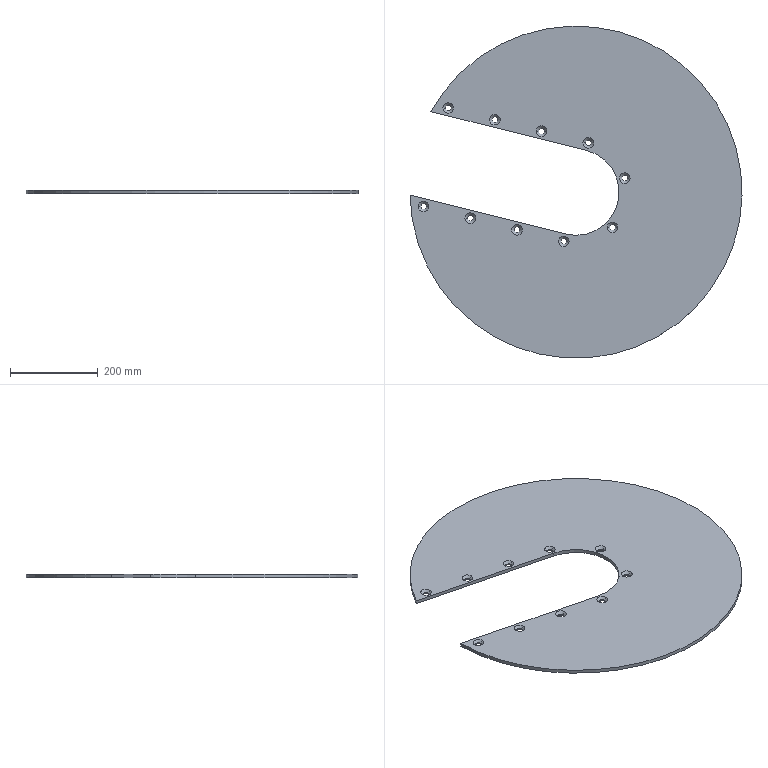Part | SolidWorks | features Extrusion 1, HoleWzd 1 | 1 solid | 46 faces | box 758.937 x 759 x 8 mm | volume 2886950 mm3 | cylinder 22 | cone 20 | plane 4 | commonest cylinder face diameters 13.5 x20 197 x1 759 x1
STEP:
#1=CARTESIAN_POINT('',(-298.885,192.389,2.55));
#2=VERTEX_POINT('',#1);
#3=CARTESIAN_POINT('',(-285.385,192.389,2.55));
#4=VERTEX_POINT('',#3);
#5=CARTESIAN_POINT('',(-292.135,192.389,2.55));
#6=DIRECTION('',(0.,0.,1.));
#7=DIRECTION('',(1.,0.,0.));
#8=AXIS2_PLACEMENT_3D('',#5,#6,#7);
#9=CIRCLE('',#8,6.75);
#10=EDGE_CURVE('',#2,#4,#9,.T.);
#11=ORIENTED_EDGE('',*,*,#10,.F.);
#12=CARTESIAN_POINT('',(-304.335,192.389,8.));
#13=VERTEX_POINT('',#12);
#14=CARTESIAN_POINT('',(-304.335,192.389,8.));
#15=DIRECTION('',(-0.7071,0.,0.7071));
#16=VECTOR('',#15,1000.);
#17=LINE('',#14,#16);
#18=EDGE_CURVE('',#2,#13,#17,.T.);
#19=ORIENTED_EDGE('',*,*,#18,.T.);
#20=CARTESIAN_POINT('',(-279.935,192.389,8.));
#21=VERTEX_POINT('',#20);
#22=CARTESIAN_POINT('',(-292.135,192.389,8.));
#23=DIRECTION('',(0.,0.,1.));
#24=DIRECTION('',(1.,0.,0.));
#25=AXIS2_PLACEMENT_3D('',#22,#23,#24);
#26=CIRCLE('',#25,12.2);
#27=EDGE_CURVE('',#13,#21,#26,.T.);
#28=ORIENTED_EDGE('',*,*,#27,.T.);
#29=CARTESIAN_POINT('',(-279.935,192.389,8.));
#30=DIRECTION('',(0.7071,0.,0.7071));
#31=VECTOR('',#30,1000.);
#32=LINE('',#29,#31);
#33=EDGE_CURVE('',#4,#21,#32,.T.);
#34=ORIENTED_EDGE('',*,*,#33,.F.);
#35=EDGE_LOOP('',(#11,#19,#28,#34));
#36=FACE_OUTER_BOUND('',#35,.T.);
#37=CARTESIAN_POINT('',(-292.135,192.389,8.));
#38=DIRECTION('',(0.,0.,1.));
#39=DIRECTION('',(1.,0.,0.));
#40=AXIS2_PLACEMENT_3D('',#37,#38,#39);
#41=CONICAL_SURFACE('',#40,12.2,0.7854);
#42=ADVANCED_FACE('',(#36),#41,.F.);
#43=CARTESIAN_POINT('',(-298.885,192.389,0.));
#44=VERTEX_POINT('',#43);
#45=CARTESIAN_POINT('',(-285.385,192.389,0.));
#46=VERTEX_POINT('',#45);
#47=CARTESIAN_POINT('',(-292.135,192.389,0.));
#48=DIRECTION('',(0.,0.,1.));
#49=DIRECTION('',(1.,0.,0.));
#50=AXIS2_PLACEMENT_3D('',#47,#48,#49);
#51=CIRCLE('',#50,6.75);
#52=EDGE_CURVE('',#44,#46,#51,.T.);
#53=ORIENTED_EDGE('',*,*,#52,.F.);
#54=CARTESIAN_POINT('',(-298.885,192.389,8.));
#55=DIRECTION('',(0.,0.,1.));
#56=VECTOR('',#55,1000.);
#57=LINE('',#54,#56);
#58=EDGE_CURVE('',#44,#2,#57,.T.);
#59=ORIENTED_EDGE('',*,*,#58,.T.);
#60=ORIENTED_EDGE('',*,*,#10,.T.);
#61=CARTESIAN_POINT('',(-285.385,192.389,8.));
#62=DIRECTION('',(0.,0.,1.));
#63=VECTOR('',#62,1000.);
#64=LINE('',#61,#63);
#65=EDGE_CURVE('',#46,#4,#64,.T.);
#66=ORIENTED_EDGE('',*,*,#65,.F.);
#67=EDGE_LOOP('',(#53,#59,#60,#66));
#68=FACE_OUTER_BOUND('',#67,.T.);
#69=CARTESIAN_POINT('',(-292.135,192.389,8.));
#70=DIRECTION('',(0.,0.,1.));
#71=DIRECTION('',(1.,0.,0.));
#72=AXIS2_PLACEMENT_3D('',#69,#70,#71);
#73=CYLINDRICAL_SURFACE('',#72,6.75);
#74=ADVANCED_FACE('',(#68),#73,.F.);
#75=CARTESIAN_POINT('',(-192.152,165.777,2.55));
#76=VERTEX_POINT('',#75);
#77=CARTESIAN_POINT('',(-178.652,165.777,2.55));
#78=VERTEX_POINT('',#77);
#79=CARTESIAN_POINT('',(-185.402,165.777,2.55));
#80=DIRECTION('',(0.,0.,1.));
#81=DIRECTION('',(1.,0.,0.));
#82=AXIS2_PLACEMENT_3D('',#79,#80,#81);
#83=CIRCLE('',#82,6.75);
#84=EDGE_CURVE('',#76,#78,#83,.T.);
#85=ORIENTED_EDGE('',*,*,#84,.F.);
#86=CARTESIAN_POINT('',(-197.602,165.777,8.));
#87=VERTEX_POINT('',#86);
#88=CARTESIAN_POINT('',(-197.602,165.777,8.));
#89=DIRECTION('',(-0.7071,0.,0.7071));
#90=VECTOR('',#89,1000.);
#91=LINE('',#88,#90);
#92=EDGE_CURVE('',#76,#87,#91,.T.);
#93=ORIENTED_EDGE('',*,*,#92,.T.);
#94=CARTESIAN_POINT('',(-173.202,165.777,8.));
#95=VERTEX_POINT('',#94);
#96=CARTESIAN_POINT('',(-185.402,165.777,8.));
#97=DIRECTION('',(0.,0.,1.));
#98=DIRECTION('',(1.,0.,0.));
#99=AXIS2_PLACEMENT_3D('',#96,#97,#98);
#100=CIRCLE('',#99,12.2);
#101=EDGE_CURVE('',#87,#95,#100,.T.);
#102=ORIENTED_EDGE('',*,*,#101,.T.);
#103=CARTESIAN_POINT('',(-173.202,165.777,8.));
#104=DIRECTION('',(0.7071,0.,0.7071));
#105=VECTOR('',#104,1000.);
#106=LINE('',#103,#105);
#107=EDGE_CURVE('',#78,#95,#106,.T.);
#108=ORIENTED_EDGE('',*,*,#107,.F.);
#109=EDGE_LOOP('',(#85,#93,#102,#108));
#110=FACE_OUTER_BOUND('',#109,.T.);
#111=CARTESIAN_POINT('',(-185.402,165.777,8.));
#112=DIRECTION('',(0.,0.,1.));
#113=DIRECTION('',(1.,0.,0.));
#114=AXIS2_PLACEMENT_3D('',#111,#112,#113);
#115=CONICAL_SURFACE('',#114,12.2,0.7854);
#116=ADVANCED_FACE('',(#110),#115,.F.);
#117=CARTESIAN_POINT('',(-192.152,165.777,0.));
#118=VERTEX_POINT('',#117);
#119=CARTESIAN_POINT('',(-178.652,165.777,0.));
#120=VERTEX_POINT('',#119);
#121=CARTESIAN_POINT('',(-185.402,165.777,0.));
#122=DIRECTION('',(0.,0.,1.));
#123=DIRECTION('',(1.,0.,0.));
#124=AXIS2_PLACEMENT_3D('',#121,#122,#123);
#125=CIRCLE('',#124,6.75);
#126=EDGE_CURVE('',#118,#120,#125,.T.);
#127=ORIENTED_EDGE('',*,*,#126,.F.);
#128=CARTESIAN_POINT('',(-192.152,165.777,8.));
#129=DIRECTION('',(0.,0.,1.));
#130=VECTOR('',#129,1000.);
#131=LINE('',#128,#130);
#132=EDGE_CURVE('',#118,#76,#131,.T.);
#133=ORIENTED_EDGE('',*,*,#132,.T.);
#134=ORIENTED_EDGE('',*,*,#84,.T.);
#135=CARTESIAN_POINT('',(-178.652,165.777,8.));
#136=DIRECTION('',(0.,0.,1.));
#137=VECTOR('',#136,1000.);
#138=LINE('',#135,#137);
#139=EDGE_CURVE('',#120,#78,#138,.T.);
#140=ORIENTED_EDGE('',*,*,#139,.F.);
#141=EDGE_LOOP('',(#127,#133,#134,#140));
#142=FACE_OUTER_BOUND('',#141,.T.);
#143=CARTESIAN_POINT('',(-185.402,165.777,8.));
#144=DIRECTION('',(0.,0.,1.));
#145=DIRECTION('',(1.,0.,0.));
#146=AXIS2_PLACEMENT_3D('',#143,#144,#145);
#147=CYLINDRICAL_SURFACE('',#146,6.75);
#148=ADVANCED_FACE('',(#142),#147,.F.);
#149=CARTESIAN_POINT('',(-85.42,139.166,2.55));
#150=VERTEX_POINT('',#149);
#151=CARTESIAN_POINT('',(-71.92,139.166,2.55));
#152=VERTEX_POINT('',#151);
#153=CARTESIAN_POINT('',(-78.67,139.166,2.55));
#154=DIRECTION('',(0.,0.,1.));
#155=DIRECTION('',(1.,0.,0.));
#156=AXIS2_PLACEMENT_3D('',#153,#154,#155);
#157=CIRCLE('',#156,6.75);
#158=EDGE_CURVE('',#150,#152,#157,.T.);
#159=ORIENTED_EDGE('',*,*,#158,.F.);
#160=CARTESIAN_POINT('',(-90.87,139.166,8.));
#161=VERTEX_POINT('',#160);
#162=CARTESIAN_POINT('',(-90.87,139.166,8.));
#163=DIRECTION('',(-0.7071,0.,0.7071));
#164=VECTOR('',#163,1000.);
#165=LINE('',#162,#164);
#166=EDGE_CURVE('',#150,#161,#165,.T.);
#167=ORIENTED_EDGE('',*,*,#166,.T.);
#168=CARTESIAN_POINT('',(-66.47,139.166,8.));
#169=VERTEX_POINT('',#168);
#170=CARTESIAN_POINT('',(-78.67,139.166,8.));
#171=DIRECTION('',(0.,0.,1.));
#172=DIRECTION('',(1.,0.,0.));
#173=AXIS2_PLACEMENT_3D('',#170,#171,#172);
#174=CIRCLE('',#173,12.2);
#175=EDGE_CURVE('',#161,#169,#174,.T.);
#176=ORIENTED_EDGE('',*,*,#175,.T.);
#177=CARTESIAN_POINT('',(-66.47,139.166,8.));
#178=DIRECTION('',(0.7071,0.,0.7071));
#179=VECTOR('',#178,1000.);
#180=LINE('',#177,#179);
#181=EDGE_CURVE('',#152,#169,#180,.T.);
#182=ORIENTED_EDGE('',*,*,#181,.F.);
#183=EDGE_LOOP('',(#159,#167,#176,#182));
#184=FACE_OUTER_BOUND('',#183,.T.);
#185=CARTESIAN_POINT('',(-78.67,139.166,8.));
#186=DIRECTION('',(0.,0.,1.));
#187=DIRECTION('',(1.,0.,0.));
#188=AXIS2_PLACEMENT_3D('',#185,#186,#187);
#189=CONICAL_SURFACE('',#188,12.2,0.7854);
#190=ADVANCED_FACE('',(#184),#189,.F.);
#191=CARTESIAN_POINT('',(-85.42,139.166,0.));
#192=VERTEX_POINT('',#191);
#193=CARTESIAN_POINT('',(-71.92,139.166,0.));
#194=VERTEX_POINT('',#193);
#195=CARTESIAN_POINT('',(-78.67,139.166,0.));
#196=DIRECTION('',(0.,0.,1.));
#197=DIRECTION('',(1.,0.,0.));
#198=AXIS2_PLACEMENT_3D('',#195,#196,#197);
#199=CIRCLE('',#198,6.75);
#200=EDGE_CURVE('',#192,#194,#199,.T.);
#201=ORIENTED_EDGE('',*,*,#200,.F.);
#202=CARTESIAN_POINT('',(-85.42,139.166,8.));
#203=DIRECTION('',(0.,0.,1.));
#204=VECTOR('',#203,1000.);
#205=LINE('',#202,#204);
#206=EDGE_CURVE('',#192,#150,#205,.T.);
#207=ORIENTED_EDGE('',*,*,#206,.T.);
#208=ORIENTED_EDGE('',*,*,#158,.T.);
#209=CARTESIAN_POINT('',(-71.92,139.166,8.));
#210=DIRECTION('',(0.,0.,1.));
#211=VECTOR('',#210,1000.);
#212=LINE('',#209,#211);
#213=EDGE_CURVE('',#194,#152,#212,.T.);
#214=ORIENTED_EDGE('',*,*,#213,.F.);
#215=EDGE_LOOP('',(#201,#207,#208,#214));
#216=FACE_OUTER_BOUND('',#215,.T.);
#217=CARTESIAN_POINT('',(-78.67,139.166,8.));
#218=DIRECTION('',(0.,0.,1.));
#219=DIRECTION('',(1.,0.,0.));
#220=AXIS2_PLACEMENT_3D('',#217,#218,#219);
#221=CYLINDRICAL_SURFACE('',#220,6.75);
#222=ADVANCED_FACE('',(#216),#221,.F.);
#223=CARTESIAN_POINT('',(21.313,112.554,2.55));
#224=VERTEX_POINT('',#223);
#225=CARTESIAN_POINT('',(34.813,112.554,2.55));
#226=VERTEX_POINT('',#225);
#227=CARTESIAN_POINT('',(28.063,112.554,2.55));
#228=DIRECTION('',(0.,0.,1.));
#229=DIRECTION('',(1.,0.,0.));
#230=AXIS2_PLACEMENT_3D('',#227,#228,#229);
#231=CIRCLE('',#230,6.75);
#232=EDGE_CURVE('',#224,#226,#231,.T.);
#233=ORIENTED_EDGE('',*,*,#232,.F.);
#234=CARTESIAN_POINT('',(15.863,112.554,8.));
#235=VERTEX_POINT('',#234);
#236=CARTESIAN_POINT('',(15.863,112.554,8.));
#237=DIRECTION('',(-0.7071,0.,0.7071));
#238=VECTOR('',#237,1000.);
#239=LINE('',#236,#238);
#240=EDGE_CURVE('',#224,#235,#239,.T.);
#241=ORIENTED_EDGE('',*,*,#240,.T.);
#242=CARTESIAN_POINT('',(40.263,112.554,8.));
#243=VERTEX_POINT('',#242);
#244=CARTESIAN_POINT('',(28.063,112.554,8.));
#245=DIRECTION('',(0.,0.,1.));
#246=DIRECTION('',(1.,0.,0.));
#247=AXIS2_PLACEMENT_3D('',#244,#245,#246);
#248=CIRCLE('',#247,12.2);
#249=EDGE_CURVE('',#235,#243,#248,.T.);
#250=ORIENTED_EDGE('',*,*,#249,.T.);
#251=CARTESIAN_POINT('',(40.263,112.554,8.));
#252=DIRECTION('',(0.7071,0.,0.7071));
#253=VECTOR('',#252,1000.);
#254=LINE('',#251,#253);
#255=EDGE_CURVE('',#226,#243,#254,.T.);
#256=ORIENTED_EDGE('',*,*,#255,.F.);
#257=EDGE_LOOP('',(#233,#241,#250,#256));
#258=FACE_OUTER_BOUND('',#257,.T.);
#259=CARTESIAN_POINT('',(28.063,112.554,8.));
#260=DIRECTION('',(0.,0.,1.));
#261=DIRECTION('',(1.,0.,0.));
#262=AXIS2_PLACEMENT_3D('',#259,#260,#261);
#263=CONICAL_SURFACE('',#262,12.2,0.7854);
#264=ADVANCED_FACE('',(#258),#263,.F.);
#265=CARTESIAN_POINT('',(21.313,112.554,0.));
#266=VERTEX_POINT('',#265);
#267=CARTESIAN_POINT('',(34.813,112.554,0.));
#268=VERTEX_POINT('',#267);
#269=CARTESIAN_POINT('',(28.063,112.554,0.));
#270=DIRECTION('',(0.,0.,1.));
#271=DIRECTION('',(1.,0.,0.));
#272=AXIS2_PLACEMENT_3D('',#269,#270,#271);
#273=CIRCLE('',#272,6.75);
#274=EDGE_CURVE('',#266,#268,#273,.T.);
#275=ORIENTED_EDGE('',*,*,#274,.F.);
#276=CARTESIAN_POINT('',(21.313,112.554,8.));
#277=DIRECTION('',(0.,0.,1.));
#278=VECTOR('',#277,1000.);
#279=LINE('',#276,#278);
#280=EDGE_CURVE('',#266,#224,#279,.T.);
#281=ORIENTED_EDGE('',*,*,#280,.T.);
#282=ORIENTED_EDGE('',*,*,#232,.T.);
#283=CARTESIAN_POINT('',(34.813,112.554,8.));
#284=DIRECTION('',(0.,0.,1.));
#285=VECTOR('',#284,1000.);
#286=LINE('',#283,#285);
#287=EDGE_CURVE('',#268,#226,#286,.T.);
#288=ORIENTED_EDGE('',*,*,#287,.F.);
#289=EDGE_LOOP('',(#275,#281,#282,#288));
#290=FACE_OUTER_BOUND('',#289,.T.);
#291=CARTESIAN_POINT('',(28.063,112.554,8.));
#292=DIRECTION('',(0.,0.,1.));
#293=DIRECTION('',(1.,0.,0.));
#294=AXIS2_PLACEMENT_3D('',#291,#292,#293);
#295=CYLINDRICAL_SURFACE('',#294,6.75);
#296=ADVANCED_FACE('',(#290),#295,.F.);
#297=CARTESIAN_POINT('',(104.756,31.974,2.55));
#298=VERTEX_POINT('',#297);
#299=CARTESIAN_POINT('',(118.256,31.974,2.55));
#300=VERTEX_POINT('',#299);
#301=CARTESIAN_POINT('',(111.506,31.974,2.55));
#302=DIRECTION('',(0.,0.,1.));
#303=DIRECTION('',(1.,0.,0.));
#304=AXIS2_PLACEMENT_3D('',#301,#302,#303);
#305=CIRCLE('',#304,6.75);
#306=EDGE_CURVE('',#298,#300,#305,.T.);
#307=ORIENTED_EDGE('',*,*,#306,.F.);
#308=CARTESIAN_POINT('',(99.306,31.974,8.));
#309=VERTEX_POINT('',#308);
#310=CARTESIAN_POINT('',(99.306,31.974,8.));
#311=DIRECTION('',(-0.7071,0.,0.7071));
#312=VECTOR('',#311,1000.);
#313=LINE('',#310,#312);
#314=EDGE_CURVE('',#298,#309,#313,.T.);
#315=ORIENTED_EDGE('',*,*,#314,.T.);
#316=CARTESIAN_POINT('',(123.706,31.974,8.));
#317=VERTEX_POINT('',#316);
#318=CARTESIAN_POINT('',(111.506,31.974,8.));
#319=DIRECTION('',(0.,0.,1.));
#320=DIRECTION('',(1.,0.,0.));
#321=AXIS2_PLACEMENT_3D('',#318,#319,#320);
#322=CIRCLE('',#321,12.2);
#323=EDGE_CURVE('',#309,#317,#322,.T.);
#324=ORIENTED_EDGE('',*,*,#323,.T.);
#325=CARTESIAN_POINT('',(123.706,31.974,8.));
#326=DIRECTION('',(0.7071,0.,0.7071));
#327=VECTOR('',#326,1000.);
#328=LINE('',#325,#327);
#329=EDGE_CURVE('',#300,#317,#328,.T.);
#330=ORIENTED_EDGE('',*,*,#329,.F.);
#331=EDGE_LOOP('',(#307,#315,#324,#330));
#332=FACE_OUTER_BOUND('',#331,.T.);
#333=CARTESIAN_POINT('',(111.506,31.974,8.));
#334=DIRECTION('',(0.,0.,1.));
#335=DIRECTION('',(1.,0.,0.));
#336=AXIS2_PLACEMENT_3D('',#333,#334,#335);
#337=CONICAL_SURFACE('',#336,12.2,0.7854);
#338=ADVANCED_FACE('',(#332),#337,.F.);
#339=CARTESIAN_POINT('',(104.756,31.974,0.));
#340=VERTEX_POINT('',#339);
#341=CARTESIAN_POINT('',(118.256,31.974,0.));
#342=VERTEX_POINT('',#341);
#343=CARTESIAN_POINT('',(111.506,31.974,0.));
#344=DIRECTION('',(0.,0.,1.));
#345=DIRECTION('',(1.,0.,0.));
#346=AXIS2_PLACEMENT_3D('',#343,#344,#345);
#347=CIRCLE('',#346,6.75);
#348=EDGE_CURVE('',#340,#342,#347,.T.);
#349=ORIENTED_EDGE('',*,*,#348,.F.);
#350=CARTESIAN_POINT('',(104.756,31.974,8.));
#351=DIRECTION('',(0.,0.,1.));
#352=VECTOR('',#351,1000.);
#353=LINE('',#350,#352);
#354=EDGE_CURVE('',#340,#298,#353,.T.);
#355=ORIENTED_EDGE('',*,*,#354,.T.);
#356=ORIENTED_EDGE('',*,*,#306,.T.);
#357=CARTESIAN_POINT('',(118.256,31.974,8.));
#358=DIRECTION('',(0.,0.,1.));
#359=VECTOR('',#358,1000.);
#360=LINE('',#357,#359);
#361=EDGE_CURVE('',#342,#300,#360,.T.);
#362=ORIENTED_EDGE('',*,*,#361,.F.);
#363=EDGE_LOOP('',(#349,#355,#356,#362));
#364=FACE_OUTER_BOUND('',#363,.T.);
#365=CARTESIAN_POINT('',(111.506,31.974,8.));
#366=DIRECTION('',(0.,0.,1.));
#367=DIRECTION('',(1.,0.,0.));
#368=AXIS2_PLACEMENT_3D('',#365,#366,#367);
#369=CYLINDRICAL_SURFACE('',#368,6.75);
#370=ADVANCED_FACE('',(#364),#369,.F.);
#371=CARTESIAN_POINT('',(76.693,-80.58,2.55));
#372=VERTEX_POINT('',#371);
#373=CARTESIAN_POINT('',(90.193,-80.58,2.55));
#374=VERTEX_POINT('',#373);
#375=CARTESIAN_POINT('',(83.443,-80.58,2.55));
#376=DIRECTION('',(0.,0.,1.));
#377=DIRECTION('',(1.,0.,0.));
#378=AXIS2_PLACEMENT_3D('',#375,#376,#377);
#379=CIRCLE('',#378,6.75);
#380=EDGE_CURVE('',#372,#374,#379,.T.);
#381=ORIENTED_EDGE('',*,*,#380,.F.);
#382=CARTESIAN_POINT('',(71.243,-80.58,8.));
#383=VERTEX_POINT('',#382);
#384=CARTESIAN_POINT('',(71.243,-80.58,8.));
#385=DIRECTION('',(-0.7071,0.,0.7071));
#386=VECTOR('',#385,1000.);
#387=LINE('',#384,#386);
#388=EDGE_CURVE('',#372,#383,#387,.T.);
#389=ORIENTED_EDGE('',*,*,#388,.T.);
#390=CARTESIAN_POINT('',(95.643,-80.58,8.));
#391=VERTEX_POINT('',#390);
#392=CARTESIAN_POINT('',(83.443,-80.58,8.));
#393=DIRECTION('',(0.,0.,1.));
#394=DIRECTION('',(1.,0.,0.));
#395=AXIS2_PLACEMENT_3D('',#392,#393,#394);
#396=CIRCLE('',#395,12.2);
#397=EDGE_CURVE('',#383,#391,#396,.T.);
#398=ORIENTED_EDGE('',*,*,#397,.T.);
#399=CARTESIAN_POINT('',(95.643,-80.58,8.));
#400=DIRECTION('',(0.7071,0.,0.7071));
#401=VECTOR('',#400,1000.);
#402=LINE('',#399,#401);
#403=EDGE_CURVE('',#374,#391,#402,.T.);
#404=ORIENTED_EDGE('',*,*,#403,.F.);
#405=EDGE_LOOP('',(#381,#389,#398,#404));
#406=FACE_OUTER_BOUND('',#405,.T.);
#407=CARTESIAN_POINT('',(83.443,-80.58,8.));
#408=DIRECTION('',(0.,0.,1.));
#409=DIRECTION('',(1.,0.,0.));
#410=AXIS2_PLACEMENT_3D('',#407,#408,#409);
#411=CONICAL_SURFACE('',#410,12.2,0.7854);
#412=ADVANCED_FACE('',(#406),#411,.F.);
#413=CARTESIAN_POINT('',(76.693,-80.58,0.));
#414=VERTEX_POINT('',#413);
#415=CARTESIAN_POINT('',(90.193,-80.58,0.));
#416=VERTEX_POINT('',#415);
#417=CARTESIAN_POINT('',(83.443,-80.58,0.));
#418=DIRECTION('',(0.,0.,1.));
#419=DIRECTION('',(1.,0.,0.));
#420=AXIS2_PLACEMENT_3D('',#417,#418,#419);
#421=CIRCLE('',#420,6.75);
#422=EDGE_CURVE('',#414,#416,#421,.T.);
#423=ORIENTED_EDGE('',*,*,#422,.F.);
#424=CARTESIAN_POINT('',(76.693,-80.58,8.));
#425=DIRECTION('',(0.,0.,1.));
#426=VECTOR('',#425,1000.);
#427=LINE('',#424,#426);
#428=EDGE_CURVE('',#414,#372,#427,.T.);
#429=ORIENTED_EDGE('',*,*,#428,.T.);
#430=ORIENTED_EDGE('',*,*,#380,.T.);
#431=CARTESIAN_POINT('',(90.193,-80.58,8.));
#432=DIRECTION('',(0.,0.,1.));
#433=VECTOR('',#432,1000.);
#434=LINE('',#431,#433);
#435=EDGE_CURVE('',#416,#374,#434,.T.);
#436=ORIENTED_EDGE('',*,*,#435,.F.);
#437=EDGE_LOOP('',(#423,#429,#430,#436));
#438=FACE_OUTER_BOUND('',#437,.T.);
#439=CARTESIAN_POINT('',(83.443,-80.58,8.));
#440=DIRECTION('',(0.,0.,1.));
#441=DIRECTION('',(1.,0.,0.));
#442=AXIS2_PLACEMENT_3D('',#439,#440,#441);
#443=CYLINDRICAL_SURFACE('',#442,6.75);
#444=ADVANCED_FACE('',(#438),#443,.F.);
#445=CARTESIAN_POINT('',(-34.813,-112.554,2.55));
#446=VERTEX_POINT('',#445);
#447=CARTESIAN_POINT('',(-21.313,-112.554,2.55));
#448=VERTEX_POINT('',#447);
#449=CARTESIAN_POINT('',(-28.063,-112.554,2.55));
#450=DIRECTION('',(0.,0.,1.));
#451=DIRECTION('',(1.,0.,0.));
#452=AXIS2_PLACEMENT_3D('',#449,#450,#451);
#453=CIRCLE('',#452,6.75);
#454=EDGE_CURVE('',#446,#448,#453,.T.);
#455=ORIENTED_EDGE('',*,*,#454,.F.);
#456=CARTESIAN_POINT('',(-40.263,-112.554,8.));
#457=VERTEX_POINT('',#456);
#458=CARTESIAN_POINT('',(-40.263,-112.554,8.));
#459=DIRECTION('',(-0.7071,0.,0.7071));
#460=VECTOR('',#459,1000.);
#461=LINE('',#458,#460);
#462=EDGE_CURVE('',#446,#457,#461,.T.);
#463=ORIENTED_EDGE('',*,*,#462,.T.);
#464=CARTESIAN_POINT('',(-15.863,-112.554,8.));
#465=VERTEX_POINT('',#464);
#466=CARTESIAN_POINT('',(-28.063,-112.554,8.));
#467=DIRECTION('',(0.,0.,1.));
#468=DIRECTION('',(1.,0.,0.));
#469=AXIS2_PLACEMENT_3D('',#466,#467,#468);
#470=CIRCLE('',#469,12.2);
#471=EDGE_CURVE('',#457,#465,#470,.T.);
#472=ORIENTED_EDGE('',*,*,#471,.T.);
#473=CARTESIAN_POINT('',(-15.863,-112.554,8.));
#474=DIRECTION('',(0.7071,0.,0.7071));
#475=VECTOR('',#474,1000.);
#476=LINE('',#473,#475);
#477=EDGE_CURVE('',#448,#465,#476,.T.);
#478=ORIENTED_EDGE('',*,*,#477,.F.);
#479=EDGE_LOOP('',(#455,#463,#472,#478));
#480=FACE_OUTER_BOUND('',#479,.T.);
#481=CARTESIAN_POINT('',(-28.063,-112.554,8.));
#482=DIRECTION('',(0.,0.,1.));
#483=DIRECTION('',(1.,0.,0.));
#484=AXIS2_PLACEMENT_3D('',#481,#482,#483);
#485=CONICAL_SURFACE('',#484,12.2,0.7854);
#486=ADVANCED_FACE('',(#480),#485,.F.);
#487=CARTESIAN_POINT('',(-34.813,-112.554,0.));
#488=VERTEX_POINT('',#487);
#489=CARTESIAN_POINT('',(-21.313,-112.554,0.));
#490=VERTEX_POINT('',#489);
#491=CARTESIAN_POINT('',(-28.063,-112.554,0.));
#492=DIRECTION('',(0.,0.,1.));
#493=DIRECTION('',(1.,0.,0.));
#494=AXIS2_PLACEMENT_3D('',#491,#492,#493);
#495=CIRCLE('',#494,6.75);
#496=EDGE_CURVE('',#488,#490,#495,.T.);
#497=ORIENTED_EDGE('',*,*,#496,.F.);
#498=CARTESIAN_POINT('',(-34.813,-112.554,8.));
#499=DIRECTION('',(0.,0.,1.));
#500=VECTOR('',#499,1000.);
#501=LINE('',#498,#500);
#502=EDGE_CURVE('',#488,#446,#501,.T.);
#503=ORIENTED_EDGE('',*,*,#502,.T.);
#504=ORIENTED_EDGE('',*,*,#454,.T.);
#505=CARTESIAN_POINT('',(-21.313,-112.554,8.));
#506=DIRECTION('',(0.,0.,1.));
#507=VECTOR('',#506,1000.);
#508=LINE('',#505,#507);
#509=EDGE_CURVE('',#490,#448,#508,.T.);
#510=ORIENTED_EDGE('',*,*,#509,.F.);
#511=EDGE_LOOP('',(#497,#503,#504,#510));
#512=FACE_OUTER_BOUND('',#511,.T.);
#513=CARTESIAN_POINT('',(-28.063,-112.554,8.));
#514=DIRECTION('',(0.,0.,1.));
#515=DIRECTION('',(1.,0.,0.));
#516=AXIS2_PLACEMENT_3D('',#513,#514,#515);
#517=CYLINDRICAL_SURFACE('',#516,6.75);
#518=ADVANCED_FACE('',(#512),#517,.F.);
#519=CARTESIAN_POINT('',(-141.545,-85.943,2.55));
#520=VERTEX_POINT('',#519);
#521=CARTESIAN_POINT('',(-128.045,-85.943,2.55));
#522=VERTEX_POINT('',#521);
#523=CARTESIAN_POINT('',(-134.795,-85.943,2.55));
#524=DIRECTION('',(0.,0.,1.));
#525=DIRECTION('',(1.,0.,0.));
#526=AXIS2_PLACEMENT_3D('',#523,#524,#525);
#527=CIRCLE('',#526,6.75);
#528=EDGE_CURVE('',#520,#522,#527,.T.);
#529=ORIENTED_EDGE('',*,*,#528,.F.);
#530=CARTESIAN_POINT('',(-146.995,-85.943,8.));
#531=VERTEX_POINT('',#530);
#532=CARTESIAN_POINT('',(-146.995,-85.943,8.));
#533=DIRECTION('',(-0.7071,0.,0.7071));
#534=VECTOR('',#533,1000.);
#535=LINE('',#532,#534);
#536=EDGE_CURVE('',#520,#531,#535,.T.);
#537=ORIENTED_EDGE('',*,*,#536,.T.);
#538=CARTESIAN_POINT('',(-122.595,-85.943,8.));
#539=VERTEX_POINT('',#538);
#540=CARTESIAN_POINT('',(-134.795,-85.943,8.));
#541=DIRECTION('',(0.,0.,1.));
#542=DIRECTION('',(1.,0.,0.));
#543=AXIS2_PLACEMENT_3D('',#540,#541,#542);
#544=CIRCLE('',#543,12.2);
#545=EDGE_CURVE('',#531,#539,#544,.T.);
#546=ORIENTED_EDGE('',*,*,#545,.T.);
#547=CARTESIAN_POINT('',(-122.595,-85.943,8.));
#548=DIRECTION('',(0.7071,0.,0.7071));
#549=VECTOR('',#548,1000.);
#550=LINE('',#547,#549);
#551=EDGE_CURVE('',#522,#539,#550,.T.);
#552=ORIENTED_EDGE('',*,*,#551,.F.);
#553=EDGE_LOOP('',(#529,#537,#546,#552));
#554=FACE_OUTER_BOUND('',#553,.T.);
#555=CARTESIAN_POINT('',(-134.795,-85.943,8.));
#556=DIRECTION('',(0.,0.,1.));
#557=DIRECTION('',(1.,0.,0.));
#558=AXIS2_PLACEMENT_3D('',#555,#556,#557);
#559=CONICAL_SURFACE('',#558,12.2,0.7854);
#560=ADVANCED_FACE('',(#554),#559,.F.);
#561=CARTESIAN_POINT('',(-141.545,-85.943,0.));
#562=VERTEX_POINT('',#561);
#563=CARTESIAN_POINT('',(-128.045,-85.943,0.));
#564=VERTEX_POINT('',#563);
#565=CARTESIAN_POINT('',(-134.795,-85.943,0.));
#566=DIRECTION('',(0.,0.,1.));
#567=DIRECTION('',(1.,0.,0.));
#568=AXIS2_PLACEMENT_3D('',#565,#566,#567);
#569=CIRCLE('',#568,6.75);
#570=EDGE_CURVE('',#562,#564,#569,.T.);
#571=ORIENTED_EDGE('',*,*,#570,.F.);
#572=CARTESIAN_POINT('',(-141.545,-85.943,8.));
#573=DIRECTION('',(0.,0.,1.));
#574=VECTOR('',#573,1000.);
#575=LINE('',#572,#574);
#576=EDGE_CURVE('',#562,#520,#575,.T.);
#577=ORIENTED_EDGE('',*,*,#576,.T.);
#578=ORIENTED_EDGE('',*,*,#528,.T.);
#579=CARTESIAN_POINT('',(-128.045,-85.943,8.));
#580=DIRECTION('',(0.,0.,1.));
#581=VECTOR('',#580,1000.);
#582=LINE('',#579,#581);
#583=EDGE_CURVE('',#564,#522,#582,.T.);
#584=ORIENTED_EDGE('',*,*,#583,.F.);
#585=EDGE_LOOP('',(#571,#577,#578,#584));
#586=FACE_OUTER_BOUND('',#585,.T.);
#587=CARTESIAN_POINT('',(-134.795,-85.943,8.));
#588=DIRECTION('',(0.,0.,1.));
#589=DIRECTION('',(1.,0.,0.));
#590=AXIS2_PLACEMENT_3D('',#587,#588,#589);
#591=CYLINDRICAL_SURFACE('',#590,6.75);
#592=ADVANCED_FACE('',(#586),#591,.F.);
#593=CARTESIAN_POINT('',(-248.278,-59.331,2.55));
#594=VERTEX_POINT('',#593);
#595=CARTESIAN_POINT('',(-234.778,-59.331,2.55));
#596=VERTEX_POINT('',#595);
#597=CARTESIAN_POINT('',(-241.528,-59.331,2.55));
#598=DIRECTION('',(0.,0.,1.));
#599=DIRECTION('',(1.,0.,0.));
#600=AXIS2_PLACEMENT_3D('',#597,#598,#599);
#601=CIRCLE('',#600,6.75);
#602=EDGE_CURVE('',#594,#596,#601,.T.);
#603=ORIENTED_EDGE('',*,*,#602,.F.);
#604=CARTESIAN_POINT('',(-253.728,-59.331,8.));
#605=VERTEX_POINT('',#604);
#606=CARTESIAN_POINT('',(-253.728,-59.331,8.));
#607=DIRECTION('',(-0.7071,0.,0.7071));
#608=VECTOR('',#607,1000.);
#609=LINE('',#606,#608);
#610=EDGE_CURVE('',#594,#605,#609,.T.);
#611=ORIENTED_EDGE('',*,*,#610,.T.);
#612=CARTESIAN_POINT('',(-229.328,-59.331,8.));
#613=VERTEX_POINT('',#612);
#614=CARTESIAN_POINT('',(-241.528,-59.331,8.));
#615=DIRECTION('',(0.,0.,1.));
#616=DIRECTION('',(1.,0.,0.));
#617=AXIS2_PLACEMENT_3D('',#614,#615,#616);
#618=CIRCLE('',#617,12.2);
#619=EDGE_CURVE('',#605,#613,#618,.T.);
#620=ORIENTED_EDGE('',*,*,#619,.T.);
#621=CARTESIAN_POINT('',(-229.328,-59.331,8.));
#622=DIRECTION('',(0.7071,0.,0.7071));
#623=VECTOR('',#622,1000.);
#624=LINE('',#621,#623);
#625=EDGE_CURVE('',#596,#613,#624,.T.);
#626=ORIENTED_EDGE('',*,*,#625,.F.);
#627=EDGE_LOOP('',(#603,#611,#620,#626));
#628=FACE_OUTER_BOUND('',#627,.T.);
#629=CARTESIAN_POINT('',(-241.528,-59.331,8.));
#630=DIRECTION('',(0.,0.,1.));
#631=DIRECTION('',(1.,0.,0.));
#632=AXIS2_PLACEMENT_3D('',#629,#630,#631);
#633=CONICAL_SURFACE('',#632,12.2,0.7854);
#634=ADVANCED_FACE('',(#628),#633,.F.);
#635=CARTESIAN_POINT('',(-248.278,-59.331,0.));
#636=VERTEX_POINT('',#635);
#637=CARTESIAN_POINT('',(-234.778,-59.331,0.));
#638=VERTEX_POINT('',#637);
#639=CARTESIAN_POINT('',(-241.528,-59.331,0.));
#640=DIRECTION('',(0.,0.,1.));
#641=DIRECTION('',(1.,0.,0.));
#642=AXIS2_PLACEMENT_3D('',#639,#640,#641);
#643=CIRCLE('',#642,6.75);
#644=EDGE_CURVE('',#636,#638,#643,.T.);
#645=ORIENTED_EDGE('',*,*,#644,.F.);
#646=CARTESIAN_POINT('',(-248.278,-59.331,8.));
#647=DIRECTION('',(0.,0.,1.));
#648=VECTOR('',#647,1000.);
#649=LINE('',#646,#648);
#650=EDGE_CURVE('',#636,#594,#649,.T.);
#651=ORIENTED_EDGE('',*,*,#650,.T.);
#652=ORIENTED_EDGE('',*,*,#602,.T.);
#653=CARTESIAN_POINT('',(-234.778,-59.331,8.));
#654=DIRECTION('',(0.,0.,1.));
#655=VECTOR('',#654,1000.);
#656=LINE('',#653,#655);
#657=EDGE_CURVE('',#638,#596,#656,.T.);
#658=ORIENTED_EDGE('',*,*,#657,.F.);
#659=EDGE_LOOP('',(#645,#651,#652,#658));
#660=FACE_OUTER_BOUND('',#659,.T.);
#661=CARTESIAN_POINT('',(-241.528,-59.331,8.));
#662=DIRECTION('',(0.,0.,1.));
#663=DIRECTION('',(1.,0.,0.));
#664=AXIS2_PLACEMENT_3D('',#661,#662,#663);
#665=CYLINDRICAL_SURFACE('',#664,6.75);
#666=ADVANCED_FACE('',(#660),#665,.F.);
#667=CARTESIAN_POINT('',(-355.011,-32.72,2.55));
#668=VERTEX_POINT('',#667);
#669=CARTESIAN_POINT('',(-341.511,-32.72,2.55));
#670=VERTEX_POINT('',#669);
#671=CARTESIAN_POINT('',(-348.261,-32.72,2.55));
#672=DIRECTION('',(0.,0.,1.));
#673=DIRECTION('',(1.,0.,0.));
#674=AXIS2_PLACEMENT_3D('',#671,#672,#673);
#675=CIRCLE('',#674,6.75);
#676=EDGE_CURVE('',#668,#670,#675,.T.);
#677=ORIENTED_EDGE('',*,*,#676,.F.);
#678=CARTESIAN_POINT('',(-360.461,-32.72,8.));
#679=VERTEX_POINT('',#678);
#680=CARTESIAN_POINT('',(-360.461,-32.72,8.));
#681=DIRECTION('',(-0.7071,0.,0.7071));
#682=VECTOR('',#681,1000.);
#683=LINE('',#680,#682);
#684=EDGE_CURVE('',#668,#679,#683,.T.);
#685=ORIENTED_EDGE('',*,*,#684,.T.);
#686=CARTESIAN_POINT('',(-336.061,-32.72,8.));
#687=VERTEX_POINT('',#686);
#688=CARTESIAN_POINT('',(-348.261,-32.72,8.));
#689=DIRECTION('',(0.,0.,1.));
#690=DIRECTION('',(1.,0.,0.));
#691=AXIS2_PLACEMENT_3D('',#688,#689,#690);
#692=CIRCLE('',#691,12.2);
#693=EDGE_CURVE('',#679,#687,#692,.T.);
#694=ORIENTED_EDGE('',*,*,#693,.T.);
#695=CARTESIAN_POINT('',(-336.061,-32.72,8.));
#696=DIRECTION('',(0.7071,0.,0.7071));
#697=VECTOR('',#696,1000.);
#698=LINE('',#695,#697);
#699=EDGE_CURVE('',#670,#687,#698,.T.);
#700=ORIENTED_EDGE('',*,*,#699,.F.);
#701=EDGE_LOOP('',(#677,#685,#694,#700));
#702=FACE_OUTER_BOUND('',#701,.T.);
#703=CARTESIAN_POINT('',(-348.261,-32.72,8.));
#704=DIRECTION('',(0.,0.,1.));
#705=DIRECTION('',(1.,0.,0.));
#706=AXIS2_PLACEMENT_3D('',#703,#704,#705);
#707=CONICAL_SURFACE('',#706,12.2,0.7854);
#708=ADVANCED_FACE('',(#702),#707,.F.);
#709=CARTESIAN_POINT('',(-355.011,-32.72,0.));
#710=VERTEX_POINT('',#709);
#711=CARTESIAN_POINT('',(-341.511,-32.72,0.));
#712=VERTEX_POINT('',#711);
#713=CARTESIAN_POINT('',(-348.261,-32.72,0.));
#714=DIRECTION('',(0.,0.,1.));
#715=DIRECTION('',(1.,0.,0.));
#716=AXIS2_PLACEMENT_3D('',#713,#714,#715);
#717=CIRCLE('',#716,6.75);
#718=EDGE_CURVE('',#710,#712,#717,.T.);
#719=ORIENTED_EDGE('',*,*,#718,.F.);
#720=CARTESIAN_POINT('',(-355.011,-32.72,8.));
#721=DIRECTION('',(0.,0.,1.));
#722=VECTOR('',#721,1000.);
#723=LINE('',#720,#722);
#724=EDGE_CURVE('',#710,#668,#723,.T.);
#725=ORIENTED_EDGE('',*,*,#724,.T.);
#726=ORIENTED_EDGE('',*,*,#676,.T.);
#727=CARTESIAN_POINT('',(-341.511,-32.72,8.));
#728=DIRECTION('',(0.,0.,1.));
#729=VECTOR('',#728,1000.);
#730=LINE('',#727,#729);
#731=EDGE_CURVE('',#712,#670,#730,.T.);
#732=ORIENTED_EDGE('',*,*,#731,.F.);
#733=EDGE_LOOP('',(#719,#725,#726,#732));
#734=FACE_OUTER_BOUND('',#733,.T.);
#735=CARTESIAN_POINT('',(-348.261,-32.72,8.));
#736=DIRECTION('',(0.,0.,1.));
#737=DIRECTION('',(1.,0.,0.));
#738=AXIS2_PLACEMENT_3D('',#735,#736,#737);
#739=CYLINDRICAL_SURFACE('',#738,6.75);
#740=ADVANCED_FACE('',(#734),#739,.F.);
#741=CARTESIAN_POINT('',(23.829,95.574,0.));
#742=VERTEX_POINT('',#741);
#743=CARTESIAN_POINT('',(-23.829,-95.574,0.));
#744=VERTEX_POINT('',#743);
#745=CARTESIAN_POINT('',(0.,0.,0.));
#746=DIRECTION('',(0.,0.,-1.));
#747=DIRECTION('',(1.,0.,0.));
#748=AXIS2_PLACEMENT_3D('',#745,#746,#747);
#749=CIRCLE('',#748,98.5);
#750=EDGE_CURVE('',#742,#744,#749,.T.);
#751=ORIENTED_EDGE('',*,*,#750,.T.);
#752=CARTESIAN_POINT('',(-23.829,-95.574,8.));
#753=VERTEX_POINT('',#752);
#754=CARTESIAN_POINT('',(-23.829,-95.574,8.));
#755=DIRECTION('',(0.,0.,-1.));
#756=VECTOR('',#755,1000.);
#757=LINE('',#754,#756);
#758=EDGE_CURVE('',#753,#744,#757,.T.);
#759=ORIENTED_EDGE('',*,*,#758,.F.);
#760=CARTESIAN_POINT('',(23.829,95.574,8.));
#761=VERTEX_POINT('',#760);
#762=CARTESIAN_POINT('',(0.,0.,8.));
#763=DIRECTION('',(0.,0.,-1.));
#764=DIRECTION('',(1.,0.,0.));
#765=AXIS2_PLACEMENT_3D('',#762,#763,#764);
#766=CIRCLE('',#765,98.5);
#767=EDGE_CURVE('',#761,#753,#766,.T.);
#768=ORIENTED_EDGE('',*,*,#767,.F.);
#769=CARTESIAN_POINT('',(23.829,95.574,8.));
#770=DIRECTION('',(0.,0.,-1.));
#771=VECTOR('',#770,1000.);
#772=LINE('',#769,#771);
#773=EDGE_CURVE('',#761,#742,#772,.T.);
#774=ORIENTED_EDGE('',*,*,#773,.T.);
#775=EDGE_LOOP('',(#751,#759,#768,#774));
#776=FACE_OUTER_BOUND('',#775,.T.);
#777=CARTESIAN_POINT('',(0.,0.,8.));
#778=DIRECTION('',(0.,0.,-1.));
#779=DIRECTION('',(-1.,0.,0.));
#780=AXIS2_PLACEMENT_3D('',#777,#778,#779);
#781=CYLINDRICAL_SURFACE('',#780,98.5);
#782=ADVANCED_FACE('',(#776),#781,.F.);
#783=CARTESIAN_POINT('',(-379.437,-6.911,0.));
#784=VERTEX_POINT('',#783);
#785=CARTESIAN_POINT('',(-23.829,-95.574,0.));
#786=DIRECTION('',(-0.9703,0.2419,0.));
#787=VECTOR('',#786,1000.);
#788=LINE('',#785,#787);
#789=EDGE_CURVE('',#744,#784,#788,.T.);
#790=ORIENTED_EDGE('',*,*,#789,.T.);
#791=CARTESIAN_POINT('',(-379.437,-6.911,8.));
#792=VERTEX_POINT('',#791);
#793=CARTESIAN_POINT('',(-379.437,-6.911,8.));
#794=DIRECTION('',(0.,0.,-1.));
#795=VECTOR('',#794,1000.);
#796=LINE('',#793,#795);
#797=EDGE_CURVE('',#792,#784,#796,.T.);
#798=ORIENTED_EDGE('',*,*,#797,.F.);
#799=CARTESIAN_POINT('',(-23.829,-95.574,8.));
#800=DIRECTION('',(-0.9703,0.2419,0.));
#801=VECTOR('',#800,1000.);
#802=LINE('',#799,#801);
#803=EDGE_CURVE('',#753,#792,#802,.T.);
#804=ORIENTED_EDGE('',*,*,#803,.F.);
#805=ORIENTED_EDGE('',*,*,#758,.T.);
#806=EDGE_LOOP('',(#790,#798,#804,#805));
#807=FACE_OUTER_BOUND('',#806,.T.);
#808=CARTESIAN_POINT('',(-23.829,-95.574,8.));
#809=DIRECTION('',(-0.2419,-0.9703,0.));
#810=DIRECTION('',(0.9703,-0.2419,0.));
#811=AXIS2_PLACEMENT_3D('',#808,#809,#810);
#812=PLANE('',#811);
#813=ADVANCED_FACE('',(#807),#812,.F.);
#814=CARTESIAN_POINT('',(-331.778,184.237,0.));
#815=VERTEX_POINT('',#814);
#816=CARTESIAN_POINT('',(0.,0.,0.));
#817=DIRECTION('',(0.,0.,1.));
#818=DIRECTION('',(1.,0.,0.));
#819=AXIS2_PLACEMENT_3D('',#816,#817,#818);
#820=CIRCLE('',#819,379.5);
#821=EDGE_CURVE('',#784,#815,#820,.T.);
#822=ORIENTED_EDGE('',*,*,#821,.T.);
#823=CARTESIAN_POINT('',(-331.778,184.237,8.));
#824=VERTEX_POINT('',#823);
#825=CARTESIAN_POINT('',(-331.778,184.237,8.));
#826=DIRECTION('',(0.,0.,-1.));
#827=VECTOR('',#826,1000.);
#828=LINE('',#825,#827);
#829=EDGE_CURVE('',#824,#815,#828,.T.);
#830=ORIENTED_EDGE('',*,*,#829,.F.);
#831=CARTESIAN_POINT('',(0.,0.,8.));
#832=DIRECTION('',(0.,0.,1.));
#833=DIRECTION('',(1.,0.,0.));
#834=AXIS2_PLACEMENT_3D('',#831,#832,#833);
#835=CIRCLE('',#834,379.5);
#836=EDGE_CURVE('',#792,#824,#835,.T.);
#837=ORIENTED_EDGE('',*,*,#836,.F.);
#838=ORIENTED_EDGE('',*,*,#797,.T.);
#839=EDGE_LOOP('',(#822,#830,#837,#838));
#840=FACE_OUTER_BOUND('',#839,.T.);
#841=CARTESIAN_POINT('',(0.,0.,8.));
#842=DIRECTION('',(0.,0.,-1.));
#843=DIRECTION('',(-1.,0.,0.));
#844=AXIS2_PLACEMENT_3D('',#841,#842,#843);
#845=CYLINDRICAL_SURFACE('',#844,379.5);
#846=ADVANCED_FACE('',(#840),#845,.T.);
#847=CARTESIAN_POINT('',(23.829,95.574,0.));
#848=DIRECTION('',(0.9703,-0.2419,0.));
#849=VECTOR('',#848,1000.);
#850=LINE('',#847,#849);
#851=EDGE_CURVE('',#815,#742,#850,.T.);
#852=ORIENTED_EDGE('',*,*,#851,.T.);
#853=ORIENTED_EDGE('',*,*,#773,.F.);
#854=CARTESIAN_POINT('',(23.829,95.574,8.));
#855=DIRECTION('',(0.9703,-0.2419,0.));
#856=VECTOR('',#855,1000.);
#857=LINE('',#854,#856);
#858=EDGE_CURVE('',#824,#761,#857,.T.);
#859=ORIENTED_EDGE('',*,*,#858,.F.);
#860=ORIENTED_EDGE('',*,*,#829,.T.);
#861=EDGE_LOOP('',(#852,#853,#859,#860));
#862=FACE_OUTER_BOUND('',#861,.T.);
#863=CARTESIAN_POINT('',(23.829,95.574,8.));
#864=DIRECTION('',(0.2419,0.9703,0.));
#865=DIRECTION('',(-0.9703,0.2419,0.));
#866=AXIS2_PLACEMENT_3D('',#863,#864,#865);
#867=PLANE('',#866);
#868=ADVANCED_FACE('',(#862),#867,.F.);
#869=CARTESIAN_POINT('',(-292.135,192.389,8.));
#870=DIRECTION('',(0.,0.,1.));
#871=DIRECTION('',(1.,0.,0.));
#872=AXIS2_PLACEMENT_3D('',#869,#870,#871);
#873=CIRCLE('',#872,12.2);
#874=EDGE_CURVE('',#21,#13,#873,.T.);
#875=ORIENTED_EDGE('',*,*,#874,.F.);
#876=ORIENTED_EDGE('',*,*,#27,.F.);
#877=EDGE_LOOP('',(#875,#876));
#878=FACE_BOUND('',#877,.T.);
#879=CARTESIAN_POINT('',(-185.402,165.777,8.));
#880=DIRECTION('',(0.,0.,1.));
#881=DIRECTION('',(1.,0.,0.));
#882=AXIS2_PLACEMENT_3D('',#879,#880,#881);
#883=CIRCLE('',#882,12.2);
#884=EDGE_CURVE('',#95,#87,#883,.T.);
#885=ORIENTED_EDGE('',*,*,#884,.F.);
#886=ORIENTED_EDGE('',*,*,#101,.F.);
#887=EDGE_LOOP('',(#885,#886));
#888=FACE_BOUND('',#887,.T.);
#889=CARTESIAN_POINT('',(-78.67,139.166,8.));
#890=DIRECTION('',(0.,0.,1.));
#891=DIRECTION('',(1.,0.,0.));
#892=AXIS2_PLACEMENT_3D('',#889,#890,#891);
#893=CIRCLE('',#892,12.2);
#894=EDGE_CURVE('',#169,#161,#893,.T.);
#895=ORIENTED_EDGE('',*,*,#894,.F.);
#896=ORIENTED_EDGE('',*,*,#175,.F.);
#897=EDGE_LOOP('',(#895,#896));
#898=FACE_BOUND('',#897,.T.);
#899=CARTESIAN_POINT('',(28.063,112.554,8.));
#900=DIRECTION('',(0.,0.,1.));
#901=DIRECTION('',(1.,0.,0.));
#902=AXIS2_PLACEMENT_3D('',#899,#900,#901);
#903=CIRCLE('',#902,12.2);
#904=EDGE_CURVE('',#243,#235,#903,.T.);
#905=ORIENTED_EDGE('',*,*,#904,.F.);
#906=ORIENTED_EDGE('',*,*,#249,.F.);
#907=EDGE_LOOP('',(#905,#906));
#908=FACE_BOUND('',#907,.T.);
#909=CARTESIAN_POINT('',(111.506,31.974,8.));
#910=DIRECTION('',(0.,0.,1.));
#911=DIRECTION('',(1.,0.,0.));
#912=AXIS2_PLACEMENT_3D('',#909,#910,#911);
#913=CIRCLE('',#912,12.2);
#914=EDGE_CURVE('',#317,#309,#913,.T.);
#915=ORIENTED_EDGE('',*,*,#914,.F.);
#916=ORIENTED_EDGE('',*,*,#323,.F.);
#917=EDGE_LOOP('',(#915,#916));
#918=FACE_BOUND('',#917,.T.);
#919=CARTESIAN_POINT('',(83.443,-80.58,8.));
#920=DIRECTION('',(0.,0.,1.));
#921=DIRECTION('',(1.,0.,0.));
#922=AXIS2_PLACEMENT_3D('',#919,#920,#921);
#923=CIRCLE('',#922,12.2);
#924=EDGE_CURVE('',#391,#383,#923,.T.);
#925=ORIENTED_EDGE('',*,*,#924,.F.);
#926=ORIENTED_EDGE('',*,*,#397,.F.);
#927=EDGE_LOOP('',(#925,#926));
#928=FACE_BOUND('',#927,.T.);
#929=CARTESIAN_POINT('',(-28.063,-112.554,8.));
#930=DIRECTION('',(0.,0.,1.));
#931=DIRECTION('',(1.,0.,0.));
#932=AXIS2_PLACEMENT_3D('',#929,#930,#931);
#933=CIRCLE('',#932,12.2);
#934=EDGE_CURVE('',#465,#457,#933,.T.);
#935=ORIENTED_EDGE('',*,*,#934,.F.);
#936=ORIENTED_EDGE('',*,*,#471,.F.);
#937=EDGE_LOOP('',(#935,#936));
#938=FACE_BOUND('',#937,.T.);
#939=CARTESIAN_POINT('',(-134.795,-85.943,8.));
#940=DIRECTION('',(0.,0.,1.));
#941=DIRECTION('',(1.,0.,0.));
#942=AXIS2_PLACEMENT_3D('',#939,#940,#941);
#943=CIRCLE('',#942,12.2);
#944=EDGE_CURVE('',#539,#531,#943,.T.);
#945=ORIENTED_EDGE('',*,*,#944,.F.);
#946=ORIENTED_EDGE('',*,*,#545,.F.);
#947=EDGE_LOOP('',(#945,#946));
#948=FACE_BOUND('',#947,.T.);
#949=CARTESIAN_POINT('',(-241.528,-59.331,8.));
#950=DIRECTION('',(0.,0.,1.));
#951=DIRECTION('',(1.,0.,0.));
#952=AXIS2_PLACEMENT_3D('',#949,#950,#951);
#953=CIRCLE('',#952,12.2);
#954=EDGE_CURVE('',#613,#605,#953,.T.);
#955=ORIENTED_EDGE('',*,*,#954,.F.);
#956=ORIENTED_EDGE('',*,*,#619,.F.);
#957=EDGE_LOOP('',(#955,#956));
#958=FACE_BOUND('',#957,.T.);
#959=CARTESIAN_POINT('',(-348.261,-32.72,8.));
#960=DIRECTION('',(0.,0.,1.));
#961=DIRECTION('',(1.,0.,0.));
#962=AXIS2_PLACEMENT_3D('',#959,#960,#961);
#963=CIRCLE('',#962,12.2);
#964=EDGE_CURVE('',#687,#679,#963,.T.);
#965=ORIENTED_EDGE('',*,*,#964,.F.);
#966=ORIENTED_EDGE('',*,*,#693,.F.);
#967=EDGE_LOOP('',(#965,#966));
#968=FACE_BOUND('',#967,.T.);
#969=ORIENTED_EDGE('',*,*,#767,.T.);
#970=ORIENTED_EDGE('',*,*,#803,.T.);
#971=ORIENTED_EDGE('',*,*,#836,.T.);
#972=ORIENTED_EDGE('',*,*,#858,.T.);
#973=EDGE_LOOP('',(#969,#970,#971,#972));
#974=FACE_OUTER_BOUND('',#973,.T.);
#975=CARTESIAN_POINT('',(0.,0.,8.));
#976=DIRECTION('',(0.,0.,1.));
#977=DIRECTION('',(1.,0.,0.));
#978=AXIS2_PLACEMENT_3D('',#975,#976,#977);
#979=PLANE('',#978);
#980=ADVANCED_FACE('',(#878,#888,#898,#908,#918,#928,#938,#948,#958,#968,#974),#979,.T.);
#981=CARTESIAN_POINT('',(-292.135,192.389,0.));
#982=DIRECTION('',(0.,0.,1.));
#983=DIRECTION('',(1.,0.,0.));
#984=AXIS2_PLACEMENT_3D('',#981,#982,#983);
#985=CIRCLE('',#984,6.75);
#986=EDGE_CURVE('',#46,#44,#985,.T.);
#987=ORIENTED_EDGE('',*,*,#986,.T.);
#988=ORIENTED_EDGE('',*,*,#52,.T.);
#989=EDGE_LOOP('',(#987,#988));
#990=FACE_BOUND('',#989,.T.);
#991=CARTESIAN_POINT('',(-185.402,165.777,0.));
#992=DIRECTION('',(0.,0.,1.));
#993=DIRECTION('',(1.,0.,0.));
#994=AXIS2_PLACEMENT_3D('',#991,#992,#993);
#995=CIRCLE('',#994,6.75);
#996=EDGE_CURVE('',#120,#118,#995,.T.);
#997=ORIENTED_EDGE('',*,*,#996,.T.);
#998=ORIENTED_EDGE('',*,*,#126,.T.);
#999=EDGE_LOOP('',(#997,#998));
#1000=FACE_BOUND('',#999,.T.);
#1001=CARTESIAN_POINT('',(-78.67,139.166,0.));
#1002=DIRECTION('',(0.,0.,1.));
#1003=DIRECTION('',(1.,0.,0.));
#1004=AXIS2_PLACEMENT_3D('',#1001,#1002,#1003);
#1005=CIRCLE('',#1004,6.75);
#1006=EDGE_CURVE('',#194,#192,#1005,.T.);
#1007=ORIENTED_EDGE('',*,*,#1006,.T.);
#1008=ORIENTED_EDGE('',*,*,#200,.T.);
#1009=EDGE_LOOP('',(#1007,#1008));
#1010=FACE_BOUND('',#1009,.T.);
#1011=CARTESIAN_POINT('',(28.063,112.554,0.));
#1012=DIRECTION('',(0.,0.,1.));
#1013=DIRECTION('',(1.,0.,0.));
#1014=AXIS2_PLACEMENT_3D('',#1011,#1012,#1013);
#1015=CIRCLE('',#1014,6.75);
#1016=EDGE_CURVE('',#268,#266,#1015,.T.);
#1017=ORIENTED_EDGE('',*,*,#1016,.T.);
#1018=ORIENTED_EDGE('',*,*,#274,.T.);
#1019=EDGE_LOOP('',(#1017,#1018));
#1020=FACE_BOUND('',#1019,.T.);
#1021=CARTESIAN_POINT('',(111.506,31.974,0.));
#1022=DIRECTION('',(0.,0.,1.));
#1023=DIRECTION('',(1.,0.,0.));
#1024=AXIS2_PLACEMENT_3D('',#1021,#1022,#1023);
#1025=CIRCLE('',#1024,6.75);
#1026=EDGE_CURVE('',#342,#340,#1025,.T.);
#1027=ORIENTED_EDGE('',*,*,#1026,.T.);
#1028=ORIENTED_EDGE('',*,*,#348,.T.);
#1029=EDGE_LOOP('',(#1027,#1028));
#1030=FACE_BOUND('',#1029,.T.);
#1031=CARTESIAN_POINT('',(83.443,-80.58,0.));
#1032=DIRECTION('',(0.,0.,1.));
#1033=DIRECTION('',(1.,0.,0.));
#1034=AXIS2_PLACEMENT_3D('',#1031,#1032,#1033);
#1035=CIRCLE('',#1034,6.75);
#1036=EDGE_CURVE('',#416,#414,#1035,.T.);
#1037=ORIENTED_EDGE('',*,*,#1036,.T.);
#1038=ORIENTED_EDGE('',*,*,#422,.T.);
#1039=EDGE_LOOP('',(#1037,#1038));
#1040=FACE_BOUND('',#1039,.T.);
#1041=CARTESIAN_POINT('',(-28.063,-112.554,0.));
#1042=DIRECTION('',(0.,0.,1.));
#1043=DIRECTION('',(1.,0.,0.));
#1044=AXIS2_PLACEMENT_3D('',#1041,#1042,#1043);
#1045=CIRCLE('',#1044,6.75);
#1046=EDGE_CURVE('',#490,#488,#1045,.T.);
#1047=ORIENTED_EDGE('',*,*,#1046,.T.);
#1048=ORIENTED_EDGE('',*,*,#496,.T.);
#1049=EDGE_LOOP('',(#1047,#1048));
#1050=FACE_BOUND('',#1049,.T.);
#1051=CARTESIAN_POINT('',(-134.795,-85.943,0.));
#1052=DIRECTION('',(0.,0.,1.));
#1053=DIRECTION('',(1.,0.,0.));
#1054=AXIS2_PLACEMENT_3D('',#1051,#1052,#1053);
#1055=CIRCLE('',#1054,6.75);
#1056=EDGE_CURVE('',#564,#562,#1055,.T.);
#1057=ORIENTED_EDGE('',*,*,#1056,.T.);
#1058=ORIENTED_EDGE('',*,*,#570,.T.);
#1059=EDGE_LOOP('',(#1057,#1058));
#1060=FACE_BOUND('',#1059,.T.);
#1061=CARTESIAN_POINT('',(-241.528,-59.331,0.));
#1062=DIRECTION('',(0.,0.,1.));
#1063=DIRECTION('',(1.,0.,0.));
#1064=AXIS2_PLACEMENT_3D('',#1061,#1062,#1063);
#1065=CIRCLE('',#1064,6.75);
#1066=EDGE_CURVE('',#638,#636,#1065,.T.);
#1067=ORIENTED_EDGE('',*,*,#1066,.T.);
#1068=ORIENTED_EDGE('',*,*,#644,.T.);
#1069=EDGE_LOOP('',(#1067,#1068));
#1070=FACE_BOUND('',#1069,.T.);
#1071=CARTESIAN_POINT('',(-348.261,-32.72,0.));
#1072=DIRECTION('',(0.,0.,1.));
#1073=DIRECTION('',(1.,0.,0.));
#1074=AXIS2_PLACEMENT_3D('',#1071,#1072,#1073);
#1075=CIRCLE('',#1074,6.75);
#1076=EDGE_CURVE('',#712,#710,#1075,.T.);
#1077=ORIENTED_EDGE('',*,*,#1076,.T.);
#1078=ORIENTED_EDGE('',*,*,#718,.T.);
#1079=EDGE_LOOP('',(#1077,#1078));
#1080=FACE_BOUND('',#1079,.T.);
#1081=ORIENTED_EDGE('',*,*,#750,.F.);
#1082=ORIENTED_EDGE('',*,*,#851,.F.);
#1083=ORIENTED_EDGE('',*,*,#821,.F.);
#1084=ORIENTED_EDGE('',*,*,#789,.F.);
#1085=EDGE_LOOP('',(#1081,#1082,#1083,#1084));
#1086=FACE_OUTER_BOUND('',#1085,.T.);
#1087=CARTESIAN_POINT('',(0.,0.,0.));
#1088=DIRECTION('',(0.,0.,1.));
#1089=DIRECTION('',(1.,0.,0.));
#1090=AXIS2_PLACEMENT_3D('',#1087,#1088,#1089);
#1091=PLANE('',#1090);
#1092=ADVANCED_FACE('',(#990,#1000,#1010,#1020,#1030,#1040,#1050,#1060,#1070,#1080,#1086),#1091,.F.);
#1093=ORIENTED_EDGE('',*,*,#724,.F.);
#1094=ORIENTED_EDGE('',*,*,#1076,.F.);
#1095=ORIENTED_EDGE('',*,*,#731,.T.);
#1096=CARTESIAN_POINT('',(-348.261,-32.72,2.55));
#1097=DIRECTION('',(0.,0.,1.));
#1098=DIRECTION('',(1.,0.,0.));
#1099=AXIS2_PLACEMENT_3D('',#1096,#1097,#1098);
#1100=CIRCLE('',#1099,6.75);
#1101=EDGE_CURVE('',#670,#668,#1100,.T.);
#1102=ORIENTED_EDGE('',*,*,#1101,.T.);
#1103=EDGE_LOOP('',(#1093,#1094,#1095,#1102));
#1104=FACE_OUTER_BOUND('',#1103,.T.);
#1105=CARTESIAN_POINT('',(-348.261,-32.72,8.));
#1106=DIRECTION('',(0.,0.,1.));
#1107=DIRECTION('',(1.,0.,0.));
#1108=AXIS2_PLACEMENT_3D('',#1105,#1106,#1107);
#1109=CYLINDRICAL_SURFACE('',#1108,6.75);
#1110=ADVANCED_FACE('',(#1104),#1109,.F.);
#1111=ORIENTED_EDGE('',*,*,#684,.F.);
#1112=ORIENTED_EDGE('',*,*,#1101,.F.);
#1113=ORIENTED_EDGE('',*,*,#699,.T.);
#1114=ORIENTED_EDGE('',*,*,#964,.T.);
#1115=EDGE_LOOP('',(#1111,#1112,#1113,#1114));
#1116=FACE_OUTER_BOUND('',#1115,.T.);
#1117=CARTESIAN_POINT('',(-348.261,-32.72,8.));
#1118=DIRECTION('',(0.,0.,1.));
#1119=DIRECTION('',(1.,0.,0.));
#1120=AXIS2_PLACEMENT_3D('',#1117,#1118,#1119);
#1121=CONICAL_SURFACE('',#1120,12.2,0.7854);
#1122=ADVANCED_FACE('',(#1116),#1121,.F.);
#1123=ORIENTED_EDGE('',*,*,#650,.F.);
#1124=ORIENTED_EDGE('',*,*,#1066,.F.);
#1125=ORIENTED_EDGE('',*,*,#657,.T.);
#1126=CARTESIAN_POINT('',(-241.528,-59.331,2.55));
#1127=DIRECTION('',(0.,0.,1.));
#1128=DIRECTION('',(1.,0.,0.));
#1129=AXIS2_PLACEMENT_3D('',#1126,#1127,#1128);
#1130=CIRCLE('',#1129,6.75);
#1131=EDGE_CURVE('',#596,#594,#1130,.T.);
#1132=ORIENTED_EDGE('',*,*,#1131,.T.);
#1133=EDGE_LOOP('',(#1123,#1124,#1125,#1132));
#1134=FACE_OUTER_BOUND('',#1133,.T.);
#1135=CARTESIAN_POINT('',(-241.528,-59.331,8.));
#1136=DIRECTION('',(0.,0.,1.));
#1137=DIRECTION('',(1.,0.,0.));
#1138=AXIS2_PLACEMENT_3D('',#1135,#1136,#1137);
#1139=CYLINDRICAL_SURFACE('',#1138,6.75);
#1140=ADVANCED_FACE('',(#1134),#1139,.F.);
#1141=ORIENTED_EDGE('',*,*,#610,.F.);
#1142=ORIENTED_EDGE('',*,*,#1131,.F.);
#1143=ORIENTED_EDGE('',*,*,#625,.T.);
#1144=ORIENTED_EDGE('',*,*,#954,.T.);
#1145=EDGE_LOOP('',(#1141,#1142,#1143,#1144));
#1146=FACE_OUTER_BOUND('',#1145,.T.);
#1147=CARTESIAN_POINT('',(-241.528,-59.331,8.));
#1148=DIRECTION('',(0.,0.,1.));
#1149=DIRECTION('',(1.,0.,0.));
#1150=AXIS2_PLACEMENT_3D('',#1147,#1148,#1149);
#1151=CONICAL_SURFACE('',#1150,12.2,0.7854);
#1152=ADVANCED_FACE('',(#1146),#1151,.F.);
#1153=ORIENTED_EDGE('',*,*,#576,.F.);
#1154=ORIENTED_EDGE('',*,*,#1056,.F.);
#1155=ORIENTED_EDGE('',*,*,#583,.T.);
#1156=CARTESIAN_POINT('',(-134.795,-85.943,2.55));
#1157=DIRECTION('',(0.,0.,1.));
#1158=DIRECTION('',(1.,0.,0.));
#1159=AXIS2_PLACEMENT_3D('',#1156,#1157,#1158);
#1160=CIRCLE('',#1159,6.75);
#1161=EDGE_CURVE('',#522,#520,#1160,.T.);
#1162=ORIENTED_EDGE('',*,*,#1161,.T.);
#1163=EDGE_LOOP('',(#1153,#1154,#1155,#1162));
#1164=FACE_OUTER_BOUND('',#1163,.T.);
#1165=CARTESIAN_POINT('',(-134.795,-85.943,8.));
#1166=DIRECTION('',(0.,0.,1.));
#1167=DIRECTION('',(1.,0.,0.));
#1168=AXIS2_PLACEMENT_3D('',#1165,#1166,#1167);
#1169=CYLINDRICAL_SURFACE('',#1168,6.75);
#1170=ADVANCED_FACE('',(#1164),#1169,.F.);
#1171=ORIENTED_EDGE('',*,*,#536,.F.);
#1172=ORIENTED_EDGE('',*,*,#1161,.F.);
#1173=ORIENTED_EDGE('',*,*,#551,.T.);
#1174=ORIENTED_EDGE('',*,*,#944,.T.);
#1175=EDGE_LOOP('',(#1171,#1172,#1173,#1174));
#1176=FACE_OUTER_BOUND('',#1175,.T.);
#1177=CARTESIAN_POINT('',(-134.795,-85.943,8.));
#1178=DIRECTION('',(0.,0.,1.));
#1179=DIRECTION('',(1.,0.,0.));
#1180=AXIS2_PLACEMENT_3D('',#1177,#1178,#1179);
#1181=CONICAL_SURFACE('',#1180,12.2,0.7854);
#1182=ADVANCED_FACE('',(#1176),#1181,.F.);
#1183=ORIENTED_EDGE('',*,*,#502,.F.);
#1184=ORIENTED_EDGE('',*,*,#1046,.F.);
#1185=ORIENTED_EDGE('',*,*,#509,.T.);
#1186=CARTESIAN_POINT('',(-28.063,-112.554,2.55));
#1187=DIRECTION('',(0.,0.,1.));
#1188=DIRECTION('',(1.,0.,0.));
#1189=AXIS2_PLACEMENT_3D('',#1186,#1187,#1188);
#1190=CIRCLE('',#1189,6.75);
#1191=EDGE_CURVE('',#448,#446,#1190,.T.);
#1192=ORIENTED_EDGE('',*,*,#1191,.T.);
#1193=EDGE_LOOP('',(#1183,#1184,#1185,#1192));
#1194=FACE_OUTER_BOUND('',#1193,.T.);
#1195=CARTESIAN_POINT('',(-28.063,-112.554,8.));
#1196=DIRECTION('',(0.,0.,1.));
#1197=DIRECTION('',(1.,0.,0.));
#1198=AXIS2_PLACEMENT_3D('',#1195,#1196,#1197);
#1199=CYLINDRICAL_SURFACE('',#1198,6.75);
#1200=ADVANCED_FACE('',(#1194),#1199,.F.);
#1201=ORIENTED_EDGE('',*,*,#462,.F.);
#1202=ORIENTED_EDGE('',*,*,#1191,.F.);
#1203=ORIENTED_EDGE('',*,*,#477,.T.);
#1204=ORIENTED_EDGE('',*,*,#934,.T.);
#1205=EDGE_LOOP('',(#1201,#1202,#1203,#1204));
#1206=FACE_OUTER_BOUND('',#1205,.T.);
#1207=CARTESIAN_POINT('',(-28.063,-112.554,8.));
#1208=DIRECTION('',(0.,0.,1.));
#1209=DIRECTION('',(1.,0.,0.));
#1210=AXIS2_PLACEMENT_3D('',#1207,#1208,#1209);
#1211=CONICAL_SURFACE('',#1210,12.2,0.7854);
#1212=ADVANCED_FACE('',(#1206),#1211,.F.);
#1213=ORIENTED_EDGE('',*,*,#428,.F.);
#1214=ORIENTED_EDGE('',*,*,#1036,.F.);
#1215=ORIENTED_EDGE('',*,*,#435,.T.);
#1216=CARTESIAN_POINT('',(83.443,-80.58,2.55));
#1217=DIRECTION('',(0.,0.,1.));
#1218=DIRECTION('',(1.,0.,0.));
#1219=AXIS2_PLACEMENT_3D('',#1216,#1217,#1218);
#1220=CIRCLE('',#1219,6.75);
#1221=EDGE_CURVE('',#374,#372,#1220,.T.);
#1222=ORIENTED_EDGE('',*,*,#1221,.T.);
#1223=EDGE_LOOP('',(#1213,#1214,#1215,#1222));
#1224=FACE_OUTER_BOUND('',#1223,.T.);
#1225=CARTESIAN_POINT('',(83.443,-80.58,8.));
#1226=DIRECTION('',(0.,0.,1.));
#1227=DIRECTION('',(1.,0.,0.));
#1228=AXIS2_PLACEMENT_3D('',#1225,#1226,#1227);
#1229=CYLINDRICAL_SURFACE('',#1228,6.75);
#1230=ADVANCED_FACE('',(#1224),#1229,.F.);
#1231=ORIENTED_EDGE('',*,*,#388,.F.);
#1232=ORIENTED_EDGE('',*,*,#1221,.F.);
#1233=ORIENTED_EDGE('',*,*,#403,.T.);
#1234=ORIENTED_EDGE('',*,*,#924,.T.);
#1235=EDGE_LOOP('',(#1231,#1232,#1233,#1234));
#1236=FACE_OUTER_BOUND('',#1235,.T.);
#1237=CARTESIAN_POINT('',(83.443,-80.58,8.));
#1238=DIRECTION('',(0.,0.,1.));
#1239=DIRECTION('',(1.,0.,0.));
#1240=AXIS2_PLACEMENT_3D('',#1237,#1238,#1239);
#1241=CONICAL_SURFACE('',#1240,12.2,0.7854);
#1242=ADVANCED_FACE('',(#1236),#1241,.F.);
#1243=ORIENTED_EDGE('',*,*,#354,.F.);
#1244=ORIENTED_EDGE('',*,*,#1026,.F.);
#1245=ORIENTED_EDGE('',*,*,#361,.T.);
#1246=CARTESIAN_POINT('',(111.506,31.974,2.55));
#1247=DIRECTION('',(0.,0.,1.));
#1248=DIRECTION('',(1.,0.,0.));
#1249=AXIS2_PLACEMENT_3D('',#1246,#1247,#1248);
#1250=CIRCLE('',#1249,6.75);
#1251=EDGE_CURVE('',#300,#298,#1250,.T.);
#1252=ORIENTED_EDGE('',*,*,#1251,.T.);
#1253=EDGE_LOOP('',(#1243,#1244,#1245,#1252));
#1254=FACE_OUTER_BOUND('',#1253,.T.);
#1255=CARTESIAN_POINT('',(111.506,31.974,8.));
#1256=DIRECTION('',(0.,0.,1.));
#1257=DIRECTION('',(1.,0.,0.));
#1258=AXIS2_PLACEMENT_3D('',#1255,#1256,#1257);
#1259=CYLINDRICAL_SURFACE('',#1258,6.75);
#1260=ADVANCED_FACE('',(#1254),#1259,.F.);
#1261=ORIENTED_EDGE('',*,*,#314,.F.);
#1262=ORIENTED_EDGE('',*,*,#1251,.F.);
#1263=ORIENTED_EDGE('',*,*,#329,.T.);
#1264=ORIENTED_EDGE('',*,*,#914,.T.);
#1265=EDGE_LOOP('',(#1261,#1262,#1263,#1264));
#1266=FACE_OUTER_BOUND('',#1265,.T.);
#1267=CARTESIAN_POINT('',(111.506,31.974,8.));
#1268=DIRECTION('',(0.,0.,1.));
#1269=DIRECTION('',(1.,0.,0.));
#1270=AXIS2_PLACEMENT_3D('',#1267,#1268,#1269);
#1271=CONICAL_SURFACE('',#1270,12.2,0.7854);
#1272=ADVANCED_FACE('',(#1266),#1271,.F.);
#1273=ORIENTED_EDGE('',*,*,#280,.F.);
#1274=ORIENTED_EDGE('',*,*,#1016,.F.);
#1275=ORIENTED_EDGE('',*,*,#287,.T.);
#1276=CARTESIAN_POINT('',(28.063,112.554,2.55));
#1277=DIRECTION('',(0.,0.,1.));
#1278=DIRECTION('',(1.,0.,0.));
#1279=AXIS2_PLACEMENT_3D('',#1276,#1277,#1278);
#1280=CIRCLE('',#1279,6.75);
#1281=EDGE_CURVE('',#226,#224,#1280,.T.);
#1282=ORIENTED_EDGE('',*,*,#1281,.T.);
#1283=EDGE_LOOP('',(#1273,#1274,#1275,#1282));
#1284=FACE_OUTER_BOUND('',#1283,.T.);
#1285=CARTESIAN_POINT('',(28.063,112.554,8.));
#1286=DIRECTION('',(0.,0.,1.));
#1287=DIRECTION('',(1.,0.,0.));
#1288=AXIS2_PLACEMENT_3D('',#1285,#1286,#1287);
#1289=CYLINDRICAL_SURFACE('',#1288,6.75);
#1290=ADVANCED_FACE('',(#1284),#1289,.F.);
#1291=ORIENTED_EDGE('',*,*,#240,.F.);
#1292=ORIENTED_EDGE('',*,*,#1281,.F.);
#1293=ORIENTED_EDGE('',*,*,#255,.T.);
#1294=ORIENTED_EDGE('',*,*,#904,.T.);
#1295=EDGE_LOOP('',(#1291,#1292,#1293,#1294));
#1296=FACE_OUTER_BOUND('',#1295,.T.);
#1297=CARTESIAN_POINT('',(28.063,112.554,8.));
#1298=DIRECTION('',(0.,0.,1.));
#1299=DIRECTION('',(1.,0.,0.));
#1300=AXIS2_PLACEMENT_3D('',#1297,#1298,#1299);
#1301=CONICAL_SURFACE('',#1300,12.2,0.7854);
#1302=ADVANCED_FACE('',(#1296),#1301,.F.);
#1303=ORIENTED_EDGE('',*,*,#206,.F.);
#1304=ORIENTED_EDGE('',*,*,#1006,.F.);
#1305=ORIENTED_EDGE('',*,*,#213,.T.);
#1306=CARTESIAN_POINT('',(-78.67,139.166,2.55));
#1307=DIRECTION('',(0.,0.,1.));
#1308=DIRECTION('',(1.,0.,0.));
#1309=AXIS2_PLACEMENT_3D('',#1306,#1307,#1308);
#1310=CIRCLE('',#1309,6.75);
#1311=EDGE_CURVE('',#152,#150,#1310,.T.);
#1312=ORIENTED_EDGE('',*,*,#1311,.T.);
#1313=EDGE_LOOP('',(#1303,#1304,#1305,#1312));
#1314=FACE_OUTER_BOUND('',#1313,.T.);
#1315=CARTESIAN_POINT('',(-78.67,139.166,8.));
#1316=DIRECTION('',(0.,0.,1.));
#1317=DIRECTION('',(1.,0.,0.));
#1318=AXIS2_PLACEMENT_3D('',#1315,#1316,#1317);
#1319=CYLINDRICAL_SURFACE('',#1318,6.75);
#1320=ADVANCED_FACE('',(#1314),#1319,.F.);
#1321=ORIENTED_EDGE('',*,*,#166,.F.);
#1322=ORIENTED_EDGE('',*,*,#1311,.F.);
#1323=ORIENTED_EDGE('',*,*,#181,.T.);
#1324=ORIENTED_EDGE('',*,*,#894,.T.);
#1325=EDGE_LOOP('',(#1321,#1322,#1323,#1324));
#1326=FACE_OUTER_BOUND('',#1325,.T.);
#1327=CARTESIAN_POINT('',(-78.67,139.166,8.));
#1328=DIRECTION('',(0.,0.,1.));
#1329=DIRECTION('',(1.,0.,0.));
#1330=AXIS2_PLACEMENT_3D('',#1327,#1328,#1329);
#1331=CONICAL_SURFACE('',#1330,12.2,0.7854);
#1332=ADVANCED_FACE('',(#1326),#1331,.F.);
#1333=ORIENTED_EDGE('',*,*,#132,.F.);
#1334=ORIENTED_EDGE('',*,*,#996,.F.);
#1335=ORIENTED_EDGE('',*,*,#139,.T.);
#1336=CARTESIAN_POINT('',(-185.402,165.777,2.55));
#1337=DIRECTION('',(0.,0.,1.));
#1338=DIRECTION('',(1.,0.,0.));
#1339=AXIS2_PLACEMENT_3D('',#1336,#1337,#1338);
#1340=CIRCLE('',#1339,6.75);
#1341=EDGE_CURVE('',#78,#76,#1340,.T.);
#1342=ORIENTED_EDGE('',*,*,#1341,.T.);
#1343=EDGE_LOOP('',(#1333,#1334,#1335,#1342));
#1344=FACE_OUTER_BOUND('',#1343,.T.);
#1345=CARTESIAN_POINT('',(-185.402,165.777,8.));
#1346=DIRECTION('',(0.,0.,1.));
#1347=DIRECTION('',(1.,0.,0.));
#1348=AXIS2_PLACEMENT_3D('',#1345,#1346,#1347);
#1349=CYLINDRICAL_SURFACE('',#1348,6.75);
#1350=ADVANCED_FACE('',(#1344),#1349,.F.);
#1351=ORIENTED_EDGE('',*,*,#92,.F.);
#1352=ORIENTED_EDGE('',*,*,#1341,.F.);
#1353=ORIENTED_EDGE('',*,*,#107,.T.);
#1354=ORIENTED_EDGE('',*,*,#884,.T.);
#1355=EDGE_LOOP('',(#1351,#1352,#1353,#1354));
#1356=FACE_OUTER_BOUND('',#1355,.T.);
#1357=CARTESIAN_POINT('',(-185.402,165.777,8.));
#1358=DIRECTION('',(0.,0.,1.));
#1359=DIRECTION('',(1.,0.,0.));
#1360=AXIS2_PLACEMENT_3D('',#1357,#1358,#1359);
#1361=CONICAL_SURFACE('',#1360,12.2,0.7854);
#1362=ADVANCED_FACE('',(#1356),#1361,.F.);
#1363=ORIENTED_EDGE('',*,*,#58,.F.);
#1364=ORIENTED_EDGE('',*,*,#986,.F.);
#1365=ORIENTED_EDGE('',*,*,#65,.T.);
#1366=CARTESIAN_POINT('',(-292.135,192.389,2.55));
#1367=DIRECTION('',(0.,0.,1.));
#1368=DIRECTION('',(1.,0.,0.));
#1369=AXIS2_PLACEMENT_3D('',#1366,#1367,#1368);
#1370=CIRCLE('',#1369,6.75);
#1371=EDGE_CURVE('',#4,#2,#1370,.T.);
#1372=ORIENTED_EDGE('',*,*,#1371,.T.);
#1373=EDGE_LOOP('',(#1363,#1364,#1365,#1372));
#1374=FACE_OUTER_BOUND('',#1373,.T.);
#1375=CARTESIAN_POINT('',(-292.135,192.389,8.));
#1376=DIRECTION('',(0.,0.,1.));
#1377=DIRECTION('',(1.,0.,0.));
#1378=AXIS2_PLACEMENT_3D('',#1375,#1376,#1377);
#1379=CYLINDRICAL_SURFACE('',#1378,6.75);
#1380=ADVANCED_FACE('',(#1374),#1379,.F.);
#1381=ORIENTED_EDGE('',*,*,#18,.F.);
#1382=ORIENTED_EDGE('',*,*,#1371,.F.);
#1383=ORIENTED_EDGE('',*,*,#33,.T.);
#1384=ORIENTED_EDGE('',*,*,#874,.T.);
#1385=EDGE_LOOP('',(#1381,#1382,#1383,#1384));
#1386=FACE_OUTER_BOUND('',#1385,.T.);
#1387=CARTESIAN_POINT('',(-292.135,192.389,8.));
#1388=DIRECTION('',(0.,0.,1.));
#1389=DIRECTION('',(1.,0.,0.));
#1390=AXIS2_PLACEMENT_3D('',#1387,#1388,#1389);
#1391=CONICAL_SURFACE('',#1390,12.2,0.7854);
#1392=ADVANCED_FACE('',(#1386),#1391,.F.);
#1393=CLOSED_SHELL('',(#42,#74,#116,#148,#190,#222,#264,#296,#338,#370,#412,#444,#486,#518,#560,#592,#634,#666,#708,#740,#782,#813,#846,#868,#980,#1092,#1110,#1122,#1140,#1152,#1170,#1182,#1200,#1212,#1230,#1242,#1260,#1272,#1290,#1302,#1320,#1332,#1350,#1362,#1380,#1392));
#1394=MANIFOLD_SOLID_BREP('',#1393);
#1395=CARTESIAN_POINT('',(0.,0.,0.));
#1396=DIRECTION('',(0.,0.,1.));
#1397=DIRECTION('',(1.,0.,0.));
#1398=AXIS2_PLACEMENT_3D('',#1395,#1396,#1397);
#1399=(LENGTH_UNIT()NAMED_UNIT(*)SI_UNIT(.MILLI.,.METRE.));
#1400=UNCERTAINTY_MEASURE_WITH_UNIT(LENGTH_MEASURE(0.00001),#1399,'','');
#1401=(NAMED_UNIT(*)PLANE_ANGLE_UNIT()SI_UNIT($,.RADIAN.));
#1402=(NAMED_UNIT(*)SI_UNIT($,.STERADIAN.)SOLID_ANGLE_UNIT());
#1403=(GEOMETRIC_REPRESENTATION_CONTEXT(3)GLOBAL_UNCERTAINTY_ASSIGNED_CONTEXT((#1400))GLOBAL_UNIT_ASSIGNED_CONTEXT((#1399,#1401,#1402))REPRESENTATION_CONTEXT('',''));
#1404=ADVANCED_BREP_SHAPE_REPRESENTATION('',(#1394,#1398),#1403);